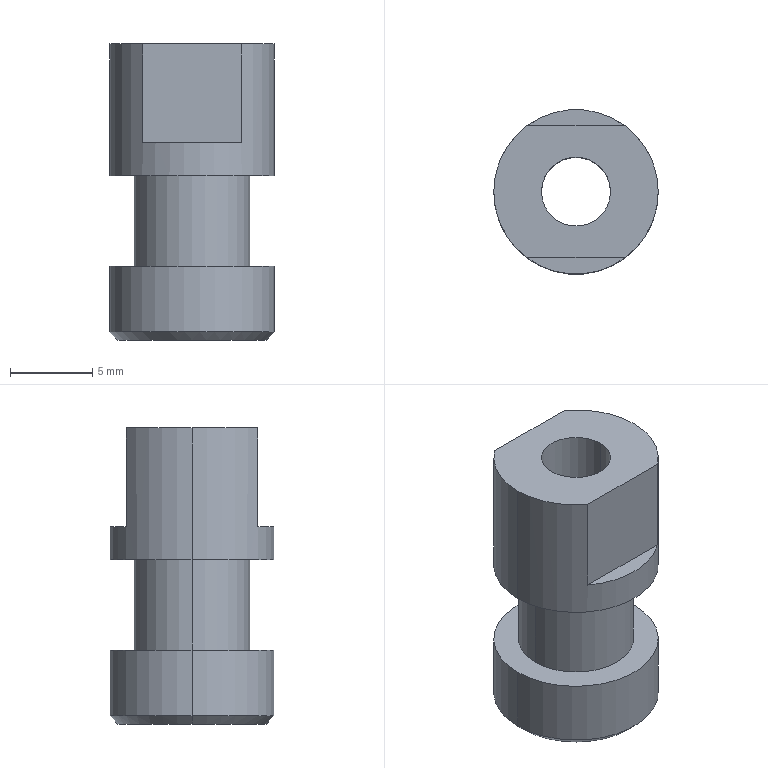Part | STEP file | 2079 Bag feed floating joint mounting | 1 solid | 18 faces | box 10 x 10 x 18 mm | volume 891.186 mm3 | cylinder 8 | plane 8 | cone 2 | commonest cylinder face diameters 10 x4 4.2 x2 7 x2
STEP:
#1=CARTESIAN_POINT('',(0.,0.,0.));
#2=DIRECTION('',(0.,0.,1.));
#3=DIRECTION('',(1.,0.,0.));
#4=AXIS2_PLACEMENT_3D('',#1,#2,#3);
#5=CARTESIAN_POINT('',(-4.5,0.,0.));
#6=VERTEX_POINT('',#5);
#7=CARTESIAN_POINT('',(4.5,0.,0.));
#8=VERTEX_POINT('',#7);
#9=CARTESIAN_POINT('',(0.,0.,0.));
#10=DIRECTION('',(0.,0.,-1.));
#11=DIRECTION('',(1.,0.,0.));
#12=AXIS2_PLACEMENT_3D('',#9,#10,#11);
#13=CIRCLE('',#12,4.5);
#14=CARTESIAN_POINT('',(0.,0.,0.5));
#15=DIRECTION('',(0.,0.,1.));
#16=DIRECTION('',(1.,0.,0.));
#17=AXIS2_PLACEMENT_3D('',#14,#15,#16);
#18=CONICAL_SURFACE('',#17,5.,0.7854);
#19=CARTESIAN_POINT('',(6.283,-0.5));
#20=DIRECTION('',(-1.,0.));
#21=VECTOR('',#20,1.);
#22=LINE('',#19,#21);
#23=(GEOMETRIC_REPRESENTATION_CONTEXT(2)PARAMETRIC_REPRESENTATION_CONTEXT()REPRESENTATION_CONTEXT('',''));
#24=DEFINITIONAL_REPRESENTATION('',(#22),#23);
#25=PCURVE('',#18,#24);
#26=CARTESIAN_POINT('',(0.,0.,0.));
#27=DIRECTION('',(0.,0.,1.));
#28=DIRECTION('',(1.,0.,0.));
#29=AXIS2_PLACEMENT_3D('',#26,#27,#28);
#30=PLANE('',#29);
#31=CARTESIAN_POINT('',(4.5,0.));
#32=CARTESIAN_POINT('',(4.5,-7.794));
#33=CARTESIAN_POINT('',(-2.25,-3.897));
#34=CARTESIAN_POINT('',(-9.,0.));
#35=CARTESIAN_POINT('',(-2.25,3.897));
#36=CARTESIAN_POINT('',(4.5,7.794));
#37=CARTESIAN_POINT('',(4.5,0.));
#38=(BOUNDED_CURVE()B_SPLINE_CURVE(2,(#31,#32,#33,#34,#35,#36,#37),.UNSPECIFIED.,.T.,.F.)B_SPLINE_CURVE_WITH_KNOTS((1,2,2,2,2,1),(-2.094,0.,2.094,4.189,6.283,8.378),.UNSPECIFIED.)CURVE()GEOMETRIC_REPRESENTATION_ITEM()RATIONAL_B_SPLINE_CURVE((1.,0.5,1.,0.5,1.,0.5,1.))REPRESENTATION_ITEM(''));
#39=(GEOMETRIC_REPRESENTATION_CONTEXT(2)PARAMETRIC_REPRESENTATION_CONTEXT()REPRESENTATION_CONTEXT('',''));
#40=DEFINITIONAL_REPRESENTATION('',(#38),#39);
#41=PCURVE('',#30,#40);
#42=SURFACE_CURVE('',#13,(#25,#41),.PCURVE_S1.);
#43=EDGE_CURVE('',#6,#8,#42,.T.);
#44=ORIENTED_EDGE('',*,*,#43,.F.);
#45=CARTESIAN_POINT('',(-5.,0.,0.5));
#46=VERTEX_POINT('',#45);
#47=CARTESIAN_POINT('',(-5.,0.,0.5));
#48=DIRECTION('',(-0.7071,0.,0.7071));
#49=VECTOR('',#48,1.);
#50=LINE('',#47,#49);
#51=CARTESIAN_POINT('',(3.142,0.));
#52=DIRECTION('',(0.,1.));
#53=VECTOR('',#52,1.);
#54=LINE('',#51,#53);
#55=(GEOMETRIC_REPRESENTATION_CONTEXT(2)PARAMETRIC_REPRESENTATION_CONTEXT()REPRESENTATION_CONTEXT('',''));
#56=DEFINITIONAL_REPRESENTATION('',(#54),#55);
#57=PCURVE('',#18,#56);
#58=CARTESIAN_POINT('',(0.,0.,0.5));
#59=DIRECTION('',(0.,0.,1.));
#60=DIRECTION('',(1.,0.,0.));
#61=AXIS2_PLACEMENT_3D('',#58,#59,#60);
#62=CONICAL_SURFACE('',#61,5.,0.7854);
#63=CARTESIAN_POINT('',(3.142,0.));
#64=DIRECTION('',(0.,1.));
#65=VECTOR('',#64,1.);
#66=LINE('',#63,#65);
#67=(GEOMETRIC_REPRESENTATION_CONTEXT(2)PARAMETRIC_REPRESENTATION_CONTEXT()REPRESENTATION_CONTEXT('',''));
#68=DEFINITIONAL_REPRESENTATION('',(#66),#67);
#69=PCURVE('',#62,#68);
#70=SURFACE_CURVE('',#50,(#57,#69),.PCURVE_S1.);
#71=EDGE_CURVE('',#6,#46,#70,.T.);
#72=ORIENTED_EDGE('',*,*,#71,.T.);
#73=CARTESIAN_POINT('',(5.,0.,0.5));
#74=VERTEX_POINT('',#73);
#75=CARTESIAN_POINT('',(0.,0.,0.5));
#76=DIRECTION('',(0.,0.,1.));
#77=DIRECTION('',(1.,0.,0.));
#78=AXIS2_PLACEMENT_3D('',#75,#76,#77);
#79=CIRCLE('',#78,5.);
#80=CARTESIAN_POINT('',(0.,0.));
#81=DIRECTION('',(1.,0.));
#82=VECTOR('',#81,1.);
#83=LINE('',#80,#82);
#84=(GEOMETRIC_REPRESENTATION_CONTEXT(2)PARAMETRIC_REPRESENTATION_CONTEXT()REPRESENTATION_CONTEXT('',''));
#85=DEFINITIONAL_REPRESENTATION('',(#83),#84);
#86=PCURVE('',#18,#85);
#87=CARTESIAN_POINT('',(0.,0.,4.5));
#88=DIRECTION('',(0.,0.,-1.));
#89=DIRECTION('',(-1.,0.,0.));
#90=AXIS2_PLACEMENT_3D('',#87,#88,#89);
#91=CYLINDRICAL_SURFACE('',#90,5.);
#92=CARTESIAN_POINT('',(3.142,4.));
#93=DIRECTION('',(-1.,0.));
#94=VECTOR('',#93,1.);
#95=LINE('',#92,#94);
#96=(GEOMETRIC_REPRESENTATION_CONTEXT(2)PARAMETRIC_REPRESENTATION_CONTEXT()REPRESENTATION_CONTEXT('',''));
#97=DEFINITIONAL_REPRESENTATION('',(#95),#96);
#98=PCURVE('',#91,#97);
#99=SURFACE_CURVE('',#79,(#86,#98),.PCURVE_S1.);
#100=EDGE_CURVE('',#74,#46,#99,.T.);
#101=ORIENTED_EDGE('',*,*,#100,.F.);
#102=CARTESIAN_POINT('',(5.,0.,0.5));
#103=DIRECTION('',(0.7071,0.,0.7071));
#104=VECTOR('',#103,1.);
#105=LINE('',#102,#104);
#106=CARTESIAN_POINT('',(0.,0.));
#107=DIRECTION('',(0.,1.));
#108=VECTOR('',#107,1.);
#109=LINE('',#106,#108);
#110=(GEOMETRIC_REPRESENTATION_CONTEXT(2)PARAMETRIC_REPRESENTATION_CONTEXT()REPRESENTATION_CONTEXT('',''));
#111=DEFINITIONAL_REPRESENTATION('',(#109),#110);
#112=PCURVE('',#18,#111);
#113=CARTESIAN_POINT('',(6.283,0.));
#114=DIRECTION('',(0.,1.));
#115=VECTOR('',#114,1.);
#116=LINE('',#113,#115);
#117=(GEOMETRIC_REPRESENTATION_CONTEXT(2)PARAMETRIC_REPRESENTATION_CONTEXT()REPRESENTATION_CONTEXT('',''));
#118=DEFINITIONAL_REPRESENTATION('',(#116),#117);
#119=PCURVE('',#62,#118);
#120=SURFACE_CURVE('',#105,(#112,#119),.PCURVE_S1.);
#121=EDGE_CURVE('',#8,#74,#120,.T.);
#122=ORIENTED_EDGE('',*,*,#121,.F.);
#123=EDGE_LOOP('',(#44,#72,#101,#122));
#124=FACE_BOUND('',#123,.T.);
#125=ADVANCED_FACE('',(#124),#18,.T.);
#126=CARTESIAN_POINT('',(2.1,0.,0.));
#127=VERTEX_POINT('',#126);
#128=CARTESIAN_POINT('',(2.1,0.,18.));
#129=VERTEX_POINT('',#128);
#130=CARTESIAN_POINT('',(2.1,0.,18.));
#131=DIRECTION('',(0.,0.,1.));
#132=VECTOR('',#131,1.);
#133=LINE('',#130,#132);
#134=CARTESIAN_POINT('',(0.,0.,18.));
#135=DIRECTION('',(0.,0.,1.));
#136=DIRECTION('',(1.,0.,0.));
#137=AXIS2_PLACEMENT_3D('',#134,#135,#136);
#138=CYLINDRICAL_SURFACE('',#137,2.1);
#139=CARTESIAN_POINT('',(6.283,0.));
#140=DIRECTION('',(0.,1.));
#141=VECTOR('',#140,1.);
#142=LINE('',#139,#141);
#143=(GEOMETRIC_REPRESENTATION_CONTEXT(2)PARAMETRIC_REPRESENTATION_CONTEXT()REPRESENTATION_CONTEXT('',''));
#144=DEFINITIONAL_REPRESENTATION('',(#142),#143);
#145=PCURVE('',#138,#144);
#146=CARTESIAN_POINT('',(0.,0.,18.));
#147=DIRECTION('',(0.,0.,1.));
#148=DIRECTION('',(1.,0.,0.));
#149=AXIS2_PLACEMENT_3D('',#146,#147,#148);
#150=CYLINDRICAL_SURFACE('',#149,2.1);
#151=CARTESIAN_POINT('',(0.,0.));
#152=DIRECTION('',(0.,1.));
#153=VECTOR('',#152,1.);
#154=LINE('',#151,#153);
#155=(GEOMETRIC_REPRESENTATION_CONTEXT(2)PARAMETRIC_REPRESENTATION_CONTEXT()REPRESENTATION_CONTEXT('',''));
#156=DEFINITIONAL_REPRESENTATION('',(#154),#155);
#157=PCURVE('',#150,#156);
#158=SURFACE_CURVE('',#133,(#145,#157),.PCURVE_S1.);
#159=EDGE_CURVE('',#127,#129,#158,.T.);
#160=ORIENTED_EDGE('',*,*,#159,.T.);
#161=CARTESIAN_POINT('',(-2.1,0.,18.));
#162=VERTEX_POINT('',#161);
#163=CARTESIAN_POINT('',(0.,0.,18.));
#164=DIRECTION('',(0.,0.,1.));
#165=DIRECTION('',(1.,0.,0.));
#166=AXIS2_PLACEMENT_3D('',#163,#164,#165);
#167=CIRCLE('',#166,2.1);
#168=CARTESIAN_POINT('',(0.,0.));
#169=DIRECTION('',(1.,0.));
#170=VECTOR('',#169,1.);
#171=LINE('',#168,#170);
#172=(GEOMETRIC_REPRESENTATION_CONTEXT(2)PARAMETRIC_REPRESENTATION_CONTEXT()REPRESENTATION_CONTEXT('',''));
#173=DEFINITIONAL_REPRESENTATION('',(#171),#172);
#174=PCURVE('',#138,#173);
#175=CARTESIAN_POINT('',(0.,0.,18.));
#176=DIRECTION('',(0.,0.,1.));
#177=DIRECTION('',(1.,0.,0.));
#178=AXIS2_PLACEMENT_3D('',#175,#176,#177);
#179=PLANE('',#178);
#180=CARTESIAN_POINT('',(0.,0.));
#181=DIRECTION('',(1.,0.));
#182=AXIS2_PLACEMENT_2D('',#180,#181);
#183=CIRCLE('',#182,2.1);
#184=(GEOMETRIC_REPRESENTATION_CONTEXT(2)PARAMETRIC_REPRESENTATION_CONTEXT()REPRESENTATION_CONTEXT('',''));
#185=DEFINITIONAL_REPRESENTATION('',(#183),#184);
#186=PCURVE('',#179,#185);
#187=SURFACE_CURVE('',#167,(#174,#186),.PCURVE_S1.);
#188=EDGE_CURVE('',#162,#129,#187,.T.);
#189=ORIENTED_EDGE('',*,*,#188,.F.);
#190=CARTESIAN_POINT('',(-2.1,0.,0.));
#191=VERTEX_POINT('',#190);
#192=CARTESIAN_POINT('',(-2.1,0.,18.));
#193=DIRECTION('',(0.,0.,1.));
#194=VECTOR('',#193,1.);
#195=LINE('',#192,#194);
#196=CARTESIAN_POINT('',(3.142,0.));
#197=DIRECTION('',(0.,1.));
#198=VECTOR('',#197,1.);
#199=LINE('',#196,#198);
#200=(GEOMETRIC_REPRESENTATION_CONTEXT(2)PARAMETRIC_REPRESENTATION_CONTEXT()REPRESENTATION_CONTEXT('',''));
#201=DEFINITIONAL_REPRESENTATION('',(#199),#200);
#202=PCURVE('',#138,#201);
#203=CARTESIAN_POINT('',(3.142,0.));
#204=DIRECTION('',(0.,1.));
#205=VECTOR('',#204,1.);
#206=LINE('',#203,#205);
#207=(GEOMETRIC_REPRESENTATION_CONTEXT(2)PARAMETRIC_REPRESENTATION_CONTEXT()REPRESENTATION_CONTEXT('',''));
#208=DEFINITIONAL_REPRESENTATION('',(#206),#207);
#209=PCURVE('',#150,#208);
#210=SURFACE_CURVE('',#195,(#202,#209),.PCURVE_S1.);
#211=EDGE_CURVE('',#191,#162,#210,.T.);
#212=ORIENTED_EDGE('',*,*,#211,.F.);
#213=CARTESIAN_POINT('',(0.,0.,0.));
#214=DIRECTION('',(0.,0.,1.));
#215=DIRECTION('',(1.,0.,0.));
#216=AXIS2_PLACEMENT_3D('',#213,#214,#215);
#217=CIRCLE('',#216,2.1);
#218=CARTESIAN_POINT('',(0.,-18.));
#219=DIRECTION('',(1.,0.));
#220=VECTOR('',#219,1.);
#221=LINE('',#218,#220);
#222=(GEOMETRIC_REPRESENTATION_CONTEXT(2)PARAMETRIC_REPRESENTATION_CONTEXT()REPRESENTATION_CONTEXT('',''));
#223=DEFINITIONAL_REPRESENTATION('',(#221),#222);
#224=PCURVE('',#138,#223);
#225=CARTESIAN_POINT('',(0.,0.));
#226=DIRECTION('',(1.,0.));
#227=AXIS2_PLACEMENT_2D('',#225,#226);
#228=CIRCLE('',#227,2.1);
#229=(GEOMETRIC_REPRESENTATION_CONTEXT(2)PARAMETRIC_REPRESENTATION_CONTEXT()REPRESENTATION_CONTEXT('',''));
#230=DEFINITIONAL_REPRESENTATION('',(#228),#229);
#231=PCURVE('',#30,#230);
#232=SURFACE_CURVE('',#217,(#224,#231),.PCURVE_S1.);
#233=EDGE_CURVE('',#191,#127,#232,.T.);
#234=ORIENTED_EDGE('',*,*,#233,.T.);
#235=EDGE_LOOP('',(#160,#189,#212,#234));
#236=FACE_BOUND('',#235,.F.);
#237=ADVANCED_FACE('',(#236),#138,.F.);
#238=CARTESIAN_POINT('',(5.,0.,18.));
#239=VERTEX_POINT('',#238);
#240=CARTESIAN_POINT('',(3.,4.,18.));
#241=VERTEX_POINT('',#240);
#242=CARTESIAN_POINT('',(0.,0.,18.));
#243=DIRECTION('',(0.,0.,1.));
#244=DIRECTION('',(1.,0.,0.));
#245=AXIS2_PLACEMENT_3D('',#242,#243,#244);
#246=CIRCLE('',#245,5.);
#247=CARTESIAN_POINT('',(0.,0.,18.));
#248=DIRECTION('',(0.,0.,-1.));
#249=DIRECTION('',(-1.,0.,0.));
#250=AXIS2_PLACEMENT_3D('',#247,#248,#249);
#251=CYLINDRICAL_SURFACE('',#250,5.);
#252=CARTESIAN_POINT('',(3.142,0.));
#253=DIRECTION('',(-1.,0.));
#254=VECTOR('',#253,1.);
#255=LINE('',#252,#254);
#256=(GEOMETRIC_REPRESENTATION_CONTEXT(2)PARAMETRIC_REPRESENTATION_CONTEXT()REPRESENTATION_CONTEXT('',''));
#257=DEFINITIONAL_REPRESENTATION('',(#255),#256);
#258=PCURVE('',#251,#257);
#259=CARTESIAN_POINT('',(0.,0.));
#260=DIRECTION('',(1.,0.));
#261=AXIS2_PLACEMENT_2D('',#259,#260);
#262=CIRCLE('',#261,5.);
#263=(GEOMETRIC_REPRESENTATION_CONTEXT(2)PARAMETRIC_REPRESENTATION_CONTEXT()REPRESENTATION_CONTEXT('',''));
#264=DEFINITIONAL_REPRESENTATION('',(#262),#263);
#265=PCURVE('',#179,#264);
#266=SURFACE_CURVE('',#246,(#258,#265),.PCURVE_S1.);
#267=EDGE_CURVE('',#239,#241,#266,.T.);
#268=ORIENTED_EDGE('',*,*,#267,.F.);
#269=CARTESIAN_POINT('',(5.,0.,10.));
#270=VERTEX_POINT('',#269);
#271=CARTESIAN_POINT('',(5.,0.,18.));
#272=DIRECTION('',(0.,0.,-1.));
#273=VECTOR('',#272,1.);
#274=LINE('',#271,#273);
#275=CARTESIAN_POINT('',(3.142,0.));
#276=DIRECTION('',(0.,1.));
#277=VECTOR('',#276,1.);
#278=LINE('',#275,#277);
#279=(GEOMETRIC_REPRESENTATION_CONTEXT(2)PARAMETRIC_REPRESENTATION_CONTEXT()REPRESENTATION_CONTEXT('',''));
#280=DEFINITIONAL_REPRESENTATION('',(#278),#279);
#281=PCURVE('',#251,#280);
#282=CARTESIAN_POINT('',(0.,0.,18.));
#283=DIRECTION('',(0.,0.,-1.));
#284=DIRECTION('',(-1.,0.,0.));
#285=AXIS2_PLACEMENT_3D('',#282,#283,#284);
#286=CYLINDRICAL_SURFACE('',#285,5.);
#287=CARTESIAN_POINT('',(3.142,0.));
#288=DIRECTION('',(0.,1.));
#289=VECTOR('',#288,1.);
#290=LINE('',#287,#289);
#291=(GEOMETRIC_REPRESENTATION_CONTEXT(2)PARAMETRIC_REPRESENTATION_CONTEXT()REPRESENTATION_CONTEXT('',''));
#292=DEFINITIONAL_REPRESENTATION('',(#290),#291);
#293=PCURVE('',#286,#292);
#294=SURFACE_CURVE('',#274,(#281,#293),.PCURVE_S1.);
#295=EDGE_CURVE('',#239,#270,#294,.T.);
#296=ORIENTED_EDGE('',*,*,#295,.T.);
#297=CARTESIAN_POINT('',(-5.,0.,10.));
#298=VERTEX_POINT('',#297);
#299=CARTESIAN_POINT('',(0.,0.,10.));
#300=DIRECTION('',(0.,0.,1.));
#301=DIRECTION('',(1.,0.,0.));
#302=AXIS2_PLACEMENT_3D('',#299,#300,#301);
#303=CIRCLE('',#302,5.);
#304=CARTESIAN_POINT('',(3.142,8.));
#305=DIRECTION('',(-1.,0.));
#306=VECTOR('',#305,1.);
#307=LINE('',#304,#306);
#308=(GEOMETRIC_REPRESENTATION_CONTEXT(2)PARAMETRIC_REPRESENTATION_CONTEXT()REPRESENTATION_CONTEXT('',''));
#309=DEFINITIONAL_REPRESENTATION('',(#307),#308);
#310=PCURVE('',#251,#309);
#311=CARTESIAN_POINT('',(0.,0.,10.));
#312=DIRECTION('',(0.,0.,1.));
#313=DIRECTION('',(1.,0.,0.));
#314=AXIS2_PLACEMENT_3D('',#311,#312,#313);
#315=PLANE('',#314);
#316=CARTESIAN_POINT('',(0.,0.));
#317=DIRECTION('',(1.,0.));
#318=AXIS2_PLACEMENT_2D('',#316,#317);
#319=CIRCLE('',#318,5.);
#320=(GEOMETRIC_REPRESENTATION_CONTEXT(2)PARAMETRIC_REPRESENTATION_CONTEXT()REPRESENTATION_CONTEXT('',''));
#321=DEFINITIONAL_REPRESENTATION('',(#319),#320);
#322=PCURVE('',#315,#321);
#323=SURFACE_CURVE('',#303,(#310,#322),.PCURVE_S1.);
#324=EDGE_CURVE('',#270,#298,#323,.T.);
#325=ORIENTED_EDGE('',*,*,#324,.T.);
#326=CARTESIAN_POINT('',(-5.,0.,18.));
#327=VERTEX_POINT('',#326);
#328=CARTESIAN_POINT('',(-5.,0.,18.));
#329=DIRECTION('',(0.,0.,-1.));
#330=VECTOR('',#329,1.);
#331=LINE('',#328,#330);
#332=CARTESIAN_POINT('',(0.,0.));
#333=DIRECTION('',(0.,1.));
#334=VECTOR('',#333,1.);
#335=LINE('',#332,#334);
#336=(GEOMETRIC_REPRESENTATION_CONTEXT(2)PARAMETRIC_REPRESENTATION_CONTEXT()REPRESENTATION_CONTEXT('',''));
#337=DEFINITIONAL_REPRESENTATION('',(#335),#336);
#338=PCURVE('',#251,#337);
#339=CARTESIAN_POINT('',(6.283,0.));
#340=DIRECTION('',(0.,1.));
#341=VECTOR('',#340,1.);
#342=LINE('',#339,#341);
#343=(GEOMETRIC_REPRESENTATION_CONTEXT(2)PARAMETRIC_REPRESENTATION_CONTEXT()REPRESENTATION_CONTEXT('',''));
#344=DEFINITIONAL_REPRESENTATION('',(#342),#343);
#345=PCURVE('',#286,#344);
#346=SURFACE_CURVE('',#331,(#338,#345),.PCURVE_S1.);
#347=EDGE_CURVE('',#327,#298,#346,.T.);
#348=ORIENTED_EDGE('',*,*,#347,.F.);
#349=CARTESIAN_POINT('',(-3.,4.,18.));
#350=VERTEX_POINT('',#349);
#351=CARTESIAN_POINT('',(0.,0.,18.));
#352=DIRECTION('',(0.,0.,1.));
#353=DIRECTION('',(1.,0.,0.));
#354=AXIS2_PLACEMENT_3D('',#351,#352,#353);
#355=CIRCLE('',#354,5.);
#356=CARTESIAN_POINT('',(3.142,0.));
#357=DIRECTION('',(-1.,0.));
#358=VECTOR('',#357,1.);
#359=LINE('',#356,#358);
#360=(GEOMETRIC_REPRESENTATION_CONTEXT(2)PARAMETRIC_REPRESENTATION_CONTEXT()REPRESENTATION_CONTEXT('',''));
#361=DEFINITIONAL_REPRESENTATION('',(#359),#360);
#362=PCURVE('',#251,#361);
#363=CARTESIAN_POINT('',(0.,0.));
#364=DIRECTION('',(1.,0.));
#365=AXIS2_PLACEMENT_2D('',#363,#364);
#366=CIRCLE('',#365,5.);
#367=(GEOMETRIC_REPRESENTATION_CONTEXT(2)PARAMETRIC_REPRESENTATION_CONTEXT()REPRESENTATION_CONTEXT('',''));
#368=DEFINITIONAL_REPRESENTATION('',(#366),#367);
#369=PCURVE('',#179,#368);
#370=SURFACE_CURVE('',#355,(#362,#369),.PCURVE_S1.);
#371=EDGE_CURVE('',#350,#327,#370,.T.);
#372=ORIENTED_EDGE('',*,*,#371,.F.);
#373=CARTESIAN_POINT('',(-3.,4.,12.));
#374=VERTEX_POINT('',#373);
#375=CARTESIAN_POINT('',(-3.,4.,18.));
#376=DIRECTION('',(0.,0.,-1.));
#377=VECTOR('',#376,1.);
#378=LINE('',#375,#377);
#379=CARTESIAN_POINT('',(0.9273,0.));
#380=DIRECTION('',(0.,1.));
#381=VECTOR('',#380,1.);
#382=LINE('',#379,#381);
#383=(GEOMETRIC_REPRESENTATION_CONTEXT(2)PARAMETRIC_REPRESENTATION_CONTEXT()REPRESENTATION_CONTEXT('',''));
#384=DEFINITIONAL_REPRESENTATION('',(#382),#383);
#385=PCURVE('',#251,#384);
#386=CARTESIAN_POINT('',(5.719,4.,12.));
#387=DIRECTION('',(0.,-1.,0.));
#388=DIRECTION('',(1.,0.,0.));
#389=AXIS2_PLACEMENT_3D('',#386,#387,#388);
#390=PLANE('',#389);
#391=CARTESIAN_POINT('',(-8.719,6.));
#392=DIRECTION('',(0.,-1.));
#393=VECTOR('',#392,1.);
#394=LINE('',#391,#393);
#395=(GEOMETRIC_REPRESENTATION_CONTEXT(2)PARAMETRIC_REPRESENTATION_CONTEXT()REPRESENTATION_CONTEXT('',''));
#396=DEFINITIONAL_REPRESENTATION('',(#394),#395);
#397=PCURVE('',#390,#396);
#398=SURFACE_CURVE('',#378,(#385,#397),.PCURVE_S1.);
#399=EDGE_CURVE('',#350,#374,#398,.T.);
#400=ORIENTED_EDGE('',*,*,#399,.T.);
#401=CARTESIAN_POINT('',(3.,4.,12.));
#402=VERTEX_POINT('',#401);
#403=CARTESIAN_POINT('',(0.,0.,12.));
#404=DIRECTION('',(0.,0.,1.));
#405=DIRECTION('',(1.,0.,0.));
#406=AXIS2_PLACEMENT_3D('',#403,#404,#405);
#407=CIRCLE('',#406,5.);
#408=CARTESIAN_POINT('',(3.142,6.));
#409=DIRECTION('',(-1.,0.));
#410=VECTOR('',#409,1.);
#411=LINE('',#408,#410);
#412=(GEOMETRIC_REPRESENTATION_CONTEXT(2)PARAMETRIC_REPRESENTATION_CONTEXT()REPRESENTATION_CONTEXT('',''));
#413=DEFINITIONAL_REPRESENTATION('',(#411),#412);
#414=PCURVE('',#251,#413);
#415=CARTESIAN_POINT('',(0.,0.,12.));
#416=DIRECTION('',(0.,0.,1.));
#417=DIRECTION('',(1.,0.,0.));
#418=AXIS2_PLACEMENT_3D('',#415,#416,#417);
#419=PLANE('',#418);
#420=CARTESIAN_POINT('',(0.,0.));
#421=DIRECTION('',(1.,0.));
#422=AXIS2_PLACEMENT_2D('',#420,#421);
#423=CIRCLE('',#422,5.);
#424=(GEOMETRIC_REPRESENTATION_CONTEXT(2)PARAMETRIC_REPRESENTATION_CONTEXT()REPRESENTATION_CONTEXT('',''));
#425=DEFINITIONAL_REPRESENTATION('',(#423),#424);
#426=PCURVE('',#419,#425);
#427=SURFACE_CURVE('',#407,(#414,#426),.PCURVE_S1.);
#428=EDGE_CURVE('',#402,#374,#427,.T.);
#429=ORIENTED_EDGE('',*,*,#428,.F.);
#430=CARTESIAN_POINT('',(3.,4.,18.));
#431=DIRECTION('',(0.,0.,1.));
#432=VECTOR('',#431,1.);
#433=LINE('',#430,#432);
#434=CARTESIAN_POINT('',(2.214,0.));
#435=DIRECTION('',(0.,-1.));
#436=VECTOR('',#435,1.);
#437=LINE('',#434,#436);
#438=(GEOMETRIC_REPRESENTATION_CONTEXT(2)PARAMETRIC_REPRESENTATION_CONTEXT()REPRESENTATION_CONTEXT('',''));
#439=DEFINITIONAL_REPRESENTATION('',(#437),#438);
#440=PCURVE('',#251,#439);
#441=CARTESIAN_POINT('',(-2.719,6.));
#442=DIRECTION('',(0.,1.));
#443=VECTOR('',#442,1.);
#444=LINE('',#441,#443);
#445=(GEOMETRIC_REPRESENTATION_CONTEXT(2)PARAMETRIC_REPRESENTATION_CONTEXT()REPRESENTATION_CONTEXT('',''));
#446=DEFINITIONAL_REPRESENTATION('',(#444),#445);
#447=PCURVE('',#390,#446);
#448=SURFACE_CURVE('',#433,(#440,#447),.PCURVE_S1.);
#449=EDGE_CURVE('',#402,#241,#448,.T.);
#450=ORIENTED_EDGE('',*,*,#449,.T.);
#451=EDGE_LOOP('',(#268,#296,#325,#348,#372,#400,#429,#450));
#452=FACE_BOUND('',#451,.T.);
#453=ADVANCED_FACE('',(#452),#251,.T.);
#454=CARTESIAN_POINT('',(3.5,0.,10.));
#455=VERTEX_POINT('',#454);
#456=CARTESIAN_POINT('',(-3.5,0.,10.));
#457=VERTEX_POINT('',#456);
#458=CARTESIAN_POINT('',(0.,0.,10.));
#459=DIRECTION('',(0.,0.,1.));
#460=DIRECTION('',(1.,0.,0.));
#461=AXIS2_PLACEMENT_3D('',#458,#459,#460);
#462=CIRCLE('',#461,3.5);
#463=CARTESIAN_POINT('',(0.,0.,10.));
#464=DIRECTION('',(0.,0.,-1.));
#465=DIRECTION('',(-1.,0.,0.));
#466=AXIS2_PLACEMENT_3D('',#463,#464,#465);
#467=CYLINDRICAL_SURFACE('',#466,3.5);
#468=CARTESIAN_POINT('',(3.142,0.));
#469=DIRECTION('',(-1.,0.));
#470=VECTOR('',#469,1.);
#471=LINE('',#468,#470);
#472=(GEOMETRIC_REPRESENTATION_CONTEXT(2)PARAMETRIC_REPRESENTATION_CONTEXT()REPRESENTATION_CONTEXT('',''));
#473=DEFINITIONAL_REPRESENTATION('',(#471),#472);
#474=PCURVE('',#467,#473);
#475=CARTESIAN_POINT('',(0.,0.));
#476=DIRECTION('',(1.,0.));
#477=AXIS2_PLACEMENT_2D('',#475,#476);
#478=CIRCLE('',#477,3.5);
#479=(GEOMETRIC_REPRESENTATION_CONTEXT(2)PARAMETRIC_REPRESENTATION_CONTEXT()REPRESENTATION_CONTEXT('',''));
#480=DEFINITIONAL_REPRESENTATION('',(#478),#479);
#481=PCURVE('',#315,#480);
#482=SURFACE_CURVE('',#462,(#474,#481),.PCURVE_S1.);
#483=EDGE_CURVE('',#455,#457,#482,.T.);
#484=ORIENTED_EDGE('',*,*,#483,.F.);
#485=CARTESIAN_POINT('',(3.5,0.,4.5));
#486=VERTEX_POINT('',#485);
#487=CARTESIAN_POINT('',(3.5,0.,10.));
#488=DIRECTION('',(0.,0.,-1.));
#489=VECTOR('',#488,1.);
#490=LINE('',#487,#489);
#491=CARTESIAN_POINT('',(3.142,0.));
#492=DIRECTION('',(0.,1.));
#493=VECTOR('',#492,1.);
#494=LINE('',#491,#493);
#495=(GEOMETRIC_REPRESENTATION_CONTEXT(2)PARAMETRIC_REPRESENTATION_CONTEXT()REPRESENTATION_CONTEXT('',''));
#496=DEFINITIONAL_REPRESENTATION('',(#494),#495);
#497=PCURVE('',#467,#496);
#498=CARTESIAN_POINT('',(0.,0.,10.));
#499=DIRECTION('',(0.,0.,-1.));
#500=DIRECTION('',(-1.,0.,0.));
#501=AXIS2_PLACEMENT_3D('',#498,#499,#500);
#502=CYLINDRICAL_SURFACE('',#501,3.5);
#503=CARTESIAN_POINT('',(3.142,0.));
#504=DIRECTION('',(0.,1.));
#505=VECTOR('',#504,1.);
#506=LINE('',#503,#505);
#507=(GEOMETRIC_REPRESENTATION_CONTEXT(2)PARAMETRIC_REPRESENTATION_CONTEXT()REPRESENTATION_CONTEXT('',''));
#508=DEFINITIONAL_REPRESENTATION('',(#506),#507);
#509=PCURVE('',#502,#508);
#510=SURFACE_CURVE('',#490,(#497,#509),.PCURVE_S1.);
#511=EDGE_CURVE('',#455,#486,#510,.T.);
#512=ORIENTED_EDGE('',*,*,#511,.T.);
#513=CARTESIAN_POINT('',(-3.5,0.,4.5));
#514=VERTEX_POINT('',#513);
#515=CARTESIAN_POINT('',(0.,0.,4.5));
#516=DIRECTION('',(0.,0.,1.));
#517=DIRECTION('',(1.,0.,0.));
#518=AXIS2_PLACEMENT_3D('',#515,#516,#517);
#519=CIRCLE('',#518,3.5);
#520=CARTESIAN_POINT('',(3.142,5.5));
#521=DIRECTION('',(-1.,0.));
#522=VECTOR('',#521,1.);
#523=LINE('',#520,#522);
#524=(GEOMETRIC_REPRESENTATION_CONTEXT(2)PARAMETRIC_REPRESENTATION_CONTEXT()REPRESENTATION_CONTEXT('',''));
#525=DEFINITIONAL_REPRESENTATION('',(#523),#524);
#526=PCURVE('',#467,#525);
#527=CARTESIAN_POINT('',(0.,0.,4.5));
#528=DIRECTION('',(0.,0.,1.));
#529=DIRECTION('',(1.,0.,0.));
#530=AXIS2_PLACEMENT_3D('',#527,#528,#529);
#531=PLANE('',#530);
#532=CARTESIAN_POINT('',(0.,0.));
#533=DIRECTION('',(1.,0.));
#534=AXIS2_PLACEMENT_2D('',#532,#533);
#535=CIRCLE('',#534,3.5);
#536=(GEOMETRIC_REPRESENTATION_CONTEXT(2)PARAMETRIC_REPRESENTATION_CONTEXT()REPRESENTATION_CONTEXT('',''));
#537=DEFINITIONAL_REPRESENTATION('',(#535),#536);
#538=PCURVE('',#531,#537);
#539=SURFACE_CURVE('',#519,(#526,#538),.PCURVE_S1.);
#540=EDGE_CURVE('',#486,#514,#539,.T.);
#541=ORIENTED_EDGE('',*,*,#540,.T.);
#542=CARTESIAN_POINT('',(-3.5,0.,10.));
#543=DIRECTION('',(0.,0.,-1.));
#544=VECTOR('',#543,1.);
#545=LINE('',#542,#544);
#546=CARTESIAN_POINT('',(0.,0.));
#547=DIRECTION('',(0.,1.));
#548=VECTOR('',#547,1.);
#549=LINE('',#546,#548);
#550=(GEOMETRIC_REPRESENTATION_CONTEXT(2)PARAMETRIC_REPRESENTATION_CONTEXT()REPRESENTATION_CONTEXT('',''));
#551=DEFINITIONAL_REPRESENTATION('',(#549),#550);
#552=PCURVE('',#467,#551);
#553=CARTESIAN_POINT('',(6.283,0.));
#554=DIRECTION('',(0.,1.));
#555=VECTOR('',#554,1.);
#556=LINE('',#553,#555);
#557=(GEOMETRIC_REPRESENTATION_CONTEXT(2)PARAMETRIC_REPRESENTATION_CONTEXT()REPRESENTATION_CONTEXT('',''));
#558=DEFINITIONAL_REPRESENTATION('',(#556),#557);
#559=PCURVE('',#502,#558);
#560=SURFACE_CURVE('',#545,(#552,#559),.PCURVE_S1.);
#561=EDGE_CURVE('',#457,#514,#560,.T.);
#562=ORIENTED_EDGE('',*,*,#561,.F.);
#563=EDGE_LOOP('',(#484,#512,#541,#562));
#564=FACE_BOUND('',#563,.T.);
#565=ADVANCED_FACE('',(#564),#467,.T.);
#566=CARTESIAN_POINT('',(5.,0.,4.5));
#567=VERTEX_POINT('',#566);
#568=CARTESIAN_POINT('',(-5.,0.,4.5));
#569=VERTEX_POINT('',#568);
#570=CARTESIAN_POINT('',(0.,0.,4.5));
#571=DIRECTION('',(0.,0.,1.));
#572=DIRECTION('',(1.,0.,0.));
#573=AXIS2_PLACEMENT_3D('',#570,#571,#572);
#574=CIRCLE('',#573,5.);
#575=CARTESIAN_POINT('',(3.142,0.));
#576=DIRECTION('',(-1.,0.));
#577=VECTOR('',#576,1.);
#578=LINE('',#575,#577);
#579=(GEOMETRIC_REPRESENTATION_CONTEXT(2)PARAMETRIC_REPRESENTATION_CONTEXT()REPRESENTATION_CONTEXT('',''));
#580=DEFINITIONAL_REPRESENTATION('',(#578),#579);
#581=PCURVE('',#91,#580);
#582=CARTESIAN_POINT('',(0.,0.));
#583=DIRECTION('',(1.,0.));
#584=AXIS2_PLACEMENT_2D('',#582,#583);
#585=CIRCLE('',#584,5.);
#586=(GEOMETRIC_REPRESENTATION_CONTEXT(2)PARAMETRIC_REPRESENTATION_CONTEXT()REPRESENTATION_CONTEXT('',''));
#587=DEFINITIONAL_REPRESENTATION('',(#585),#586);
#588=PCURVE('',#531,#587);
#589=SURFACE_CURVE('',#574,(#581,#588),.PCURVE_S1.);
#590=EDGE_CURVE('',#567,#569,#589,.T.);
#591=ORIENTED_EDGE('',*,*,#590,.F.);
#592=CARTESIAN_POINT('',(5.,0.,4.5));
#593=DIRECTION('',(0.,0.,-1.));
#594=VECTOR('',#593,1.);
#595=LINE('',#592,#594);
#596=CARTESIAN_POINT('',(3.142,0.));
#597=DIRECTION('',(0.,1.));
#598=VECTOR('',#597,1.);
#599=LINE('',#596,#598);
#600=(GEOMETRIC_REPRESENTATION_CONTEXT(2)PARAMETRIC_REPRESENTATION_CONTEXT()REPRESENTATION_CONTEXT('',''));
#601=DEFINITIONAL_REPRESENTATION('',(#599),#600);
#602=PCURVE('',#91,#601);
#603=CARTESIAN_POINT('',(0.,0.,4.5));
#604=DIRECTION('',(0.,0.,-1.));
#605=DIRECTION('',(-1.,0.,0.));
#606=AXIS2_PLACEMENT_3D('',#603,#604,#605);
#607=CYLINDRICAL_SURFACE('',#606,5.);
#608=CARTESIAN_POINT('',(3.142,0.));
#609=DIRECTION('',(0.,1.));
#610=VECTOR('',#609,1.);
#611=LINE('',#608,#610);
#612=(GEOMETRIC_REPRESENTATION_CONTEXT(2)PARAMETRIC_REPRESENTATION_CONTEXT()REPRESENTATION_CONTEXT('',''));
#613=DEFINITIONAL_REPRESENTATION('',(#611),#612);
#614=PCURVE('',#607,#613);
#615=SURFACE_CURVE('',#595,(#602,#614),.PCURVE_S1.);
#616=EDGE_CURVE('',#567,#74,#615,.T.);
#617=ORIENTED_EDGE('',*,*,#616,.T.);
#618=ORIENTED_EDGE('',*,*,#100,.T.);
#619=CARTESIAN_POINT('',(-5.,0.,4.5));
#620=DIRECTION('',(0.,0.,-1.));
#621=VECTOR('',#620,1.);
#622=LINE('',#619,#621);
#623=CARTESIAN_POINT('',(0.,0.));
#624=DIRECTION('',(0.,1.));
#625=VECTOR('',#624,1.);
#626=LINE('',#623,#625);
#627=(GEOMETRIC_REPRESENTATION_CONTEXT(2)PARAMETRIC_REPRESENTATION_CONTEXT()REPRESENTATION_CONTEXT('',''));
#628=DEFINITIONAL_REPRESENTATION('',(#626),#627);
#629=PCURVE('',#91,#628);
#630=CARTESIAN_POINT('',(6.283,0.));
#631=DIRECTION('',(0.,1.));
#632=VECTOR('',#631,1.);
#633=LINE('',#630,#632);
#634=(GEOMETRIC_REPRESENTATION_CONTEXT(2)PARAMETRIC_REPRESENTATION_CONTEXT()REPRESENTATION_CONTEXT('',''));
#635=DEFINITIONAL_REPRESENTATION('',(#633),#634);
#636=PCURVE('',#607,#635);
#637=SURFACE_CURVE('',#622,(#629,#636),.PCURVE_S1.);
#638=EDGE_CURVE('',#569,#46,#637,.T.);
#639=ORIENTED_EDGE('',*,*,#638,.F.);
#640=EDGE_LOOP('',(#591,#617,#618,#639));
#641=FACE_BOUND('',#640,.T.);
#642=ADVANCED_FACE('',(#641),#91,.T.);
#643=CARTESIAN_POINT('',(0.,0.,4.5));
#644=DIRECTION('',(0.,0.,1.));
#645=DIRECTION('',(1.,0.,0.));
#646=AXIS2_PLACEMENT_3D('',#643,#644,#645);
#647=CIRCLE('',#646,5.);
#648=CARTESIAN_POINT('',(0.,0.));
#649=DIRECTION('',(1.,0.));
#650=AXIS2_PLACEMENT_2D('',#648,#649);
#651=CIRCLE('',#650,5.);
#652=(GEOMETRIC_REPRESENTATION_CONTEXT(2)PARAMETRIC_REPRESENTATION_CONTEXT()REPRESENTATION_CONTEXT('',''));
#653=DEFINITIONAL_REPRESENTATION('',(#651),#652);
#654=PCURVE('',#531,#653);
#655=CARTESIAN_POINT('',(9.425,0.));
#656=DIRECTION('',(-1.,0.));
#657=VECTOR('',#656,1.);
#658=LINE('',#655,#657);
#659=(GEOMETRIC_REPRESENTATION_CONTEXT(2)PARAMETRIC_REPRESENTATION_CONTEXT()REPRESENTATION_CONTEXT('',''));
#660=DEFINITIONAL_REPRESENTATION('',(#658),#659);
#661=PCURVE('',#607,#660);
#662=SURFACE_CURVE('',#647,(#654,#661),.PCURVE_S1.);
#663=EDGE_CURVE('',#569,#567,#662,.T.);
#664=ORIENTED_EDGE('',*,*,#663,.T.);
#665=ORIENTED_EDGE('',*,*,#590,.T.);
#666=EDGE_LOOP('',(#664,#665));
#667=FACE_BOUND('',#666,.T.);
#668=CARTESIAN_POINT('',(0.,0.,4.5));
#669=DIRECTION('',(0.,0.,1.));
#670=DIRECTION('',(1.,0.,0.));
#671=AXIS2_PLACEMENT_3D('',#668,#669,#670);
#672=CIRCLE('',#671,3.5);
#673=CARTESIAN_POINT('',(0.,0.));
#674=DIRECTION('',(1.,0.));
#675=AXIS2_PLACEMENT_2D('',#673,#674);
#676=CIRCLE('',#675,3.5);
#677=(GEOMETRIC_REPRESENTATION_CONTEXT(2)PARAMETRIC_REPRESENTATION_CONTEXT()REPRESENTATION_CONTEXT('',''));
#678=DEFINITIONAL_REPRESENTATION('',(#676),#677);
#679=PCURVE('',#531,#678);
#680=CARTESIAN_POINT('',(9.425,5.5));
#681=DIRECTION('',(-1.,0.));
#682=VECTOR('',#681,1.);
#683=LINE('',#680,#682);
#684=(GEOMETRIC_REPRESENTATION_CONTEXT(2)PARAMETRIC_REPRESENTATION_CONTEXT()REPRESENTATION_CONTEXT('',''));
#685=DEFINITIONAL_REPRESENTATION('',(#683),#684);
#686=PCURVE('',#502,#685);
#687=SURFACE_CURVE('',#672,(#679,#686),.PCURVE_S1.);
#688=EDGE_CURVE('',#514,#486,#687,.T.);
#689=ORIENTED_EDGE('',*,*,#688,.F.);
#690=ORIENTED_EDGE('',*,*,#540,.F.);
#691=EDGE_LOOP('',(#689,#690));
#692=FACE_BOUND('',#691,.T.);
#693=ADVANCED_FACE('',(#667,#692),#531,.T.);
#694=ORIENTED_EDGE('',*,*,#616,.F.);
#695=ORIENTED_EDGE('',*,*,#663,.F.);
#696=ORIENTED_EDGE('',*,*,#638,.T.);
#697=CARTESIAN_POINT('',(0.,0.,0.5));
#698=DIRECTION('',(0.,0.,1.));
#699=DIRECTION('',(1.,0.,0.));
#700=AXIS2_PLACEMENT_3D('',#697,#698,#699);
#701=CIRCLE('',#700,5.);
#702=CARTESIAN_POINT('',(9.425,4.));
#703=DIRECTION('',(-1.,0.));
#704=VECTOR('',#703,1.);
#705=LINE('',#702,#704);
#706=(GEOMETRIC_REPRESENTATION_CONTEXT(2)PARAMETRIC_REPRESENTATION_CONTEXT()REPRESENTATION_CONTEXT('',''));
#707=DEFINITIONAL_REPRESENTATION('',(#705),#706);
#708=PCURVE('',#607,#707);
#709=CARTESIAN_POINT('',(0.,0.));
#710=DIRECTION('',(1.,0.));
#711=VECTOR('',#710,1.);
#712=LINE('',#709,#711);
#713=(GEOMETRIC_REPRESENTATION_CONTEXT(2)PARAMETRIC_REPRESENTATION_CONTEXT()REPRESENTATION_CONTEXT('',''));
#714=DEFINITIONAL_REPRESENTATION('',(#712),#713);
#715=PCURVE('',#62,#714);
#716=SURFACE_CURVE('',#701,(#708,#715),.PCURVE_S1.);
#717=EDGE_CURVE('',#46,#74,#716,.T.);
#718=ORIENTED_EDGE('',*,*,#717,.T.);
#719=EDGE_LOOP('',(#694,#695,#696,#718));
#720=FACE_BOUND('',#719,.T.);
#721=ADVANCED_FACE('',(#720),#607,.T.);
#722=CARTESIAN_POINT('',(0.,0.,0.));
#723=DIRECTION('',(0.,0.,-1.));
#724=DIRECTION('',(1.,0.,0.));
#725=AXIS2_PLACEMENT_3D('',#722,#723,#724);
#726=CIRCLE('',#725,4.5);
#727=CARTESIAN_POINT('',(4.5,0.));
#728=CARTESIAN_POINT('',(4.5,-7.794));
#729=CARTESIAN_POINT('',(-2.25,-3.897));
#730=CARTESIAN_POINT('',(-9.,0.));
#731=CARTESIAN_POINT('',(-2.25,3.897));
#732=CARTESIAN_POINT('',(4.5,7.794));
#733=CARTESIAN_POINT('',(4.5,0.));
#734=(BOUNDED_CURVE()B_SPLINE_CURVE(2,(#727,#728,#729,#730,#731,#732,#733),.UNSPECIFIED.,.T.,.F.)B_SPLINE_CURVE_WITH_KNOTS((1,2,2,2,2,1),(-2.094,0.,2.094,4.189,6.283,8.378),.UNSPECIFIED.)CURVE()GEOMETRIC_REPRESENTATION_ITEM()RATIONAL_B_SPLINE_CURVE((1.,0.5,1.,0.5,1.,0.5,1.))REPRESENTATION_ITEM(''));
#735=(GEOMETRIC_REPRESENTATION_CONTEXT(2)PARAMETRIC_REPRESENTATION_CONTEXT()REPRESENTATION_CONTEXT('',''));
#736=DEFINITIONAL_REPRESENTATION('',(#734),#735);
#737=PCURVE('',#30,#736);
#738=CARTESIAN_POINT('',(6.283,-0.5));
#739=DIRECTION('',(-1.,0.));
#740=VECTOR('',#739,1.);
#741=LINE('',#738,#740);
#742=(GEOMETRIC_REPRESENTATION_CONTEXT(2)PARAMETRIC_REPRESENTATION_CONTEXT()REPRESENTATION_CONTEXT('',''));
#743=DEFINITIONAL_REPRESENTATION('',(#741),#742);
#744=PCURVE('',#62,#743);
#745=SURFACE_CURVE('',#726,(#737,#744),.PCURVE_S1.);
#746=EDGE_CURVE('',#8,#6,#745,.T.);
#747=ORIENTED_EDGE('',*,*,#746,.T.);
#748=ORIENTED_EDGE('',*,*,#43,.T.);
#749=EDGE_LOOP('',(#747,#748));
#750=FACE_BOUND('',#749,.T.);
#751=CARTESIAN_POINT('',(0.,0.,0.));
#752=DIRECTION('',(0.,0.,1.));
#753=DIRECTION('',(1.,0.,0.));
#754=AXIS2_PLACEMENT_3D('',#751,#752,#753);
#755=CIRCLE('',#754,2.1);
#756=CARTESIAN_POINT('',(0.,0.));
#757=DIRECTION('',(1.,0.));
#758=AXIS2_PLACEMENT_2D('',#756,#757);
#759=CIRCLE('',#758,2.1);
#760=(GEOMETRIC_REPRESENTATION_CONTEXT(2)PARAMETRIC_REPRESENTATION_CONTEXT()REPRESENTATION_CONTEXT('',''));
#761=DEFINITIONAL_REPRESENTATION('',(#759),#760);
#762=PCURVE('',#30,#761);
#763=CARTESIAN_POINT('',(0.,-18.));
#764=DIRECTION('',(1.,0.));
#765=VECTOR('',#764,1.);
#766=LINE('',#763,#765);
#767=(GEOMETRIC_REPRESENTATION_CONTEXT(2)PARAMETRIC_REPRESENTATION_CONTEXT()REPRESENTATION_CONTEXT('',''));
#768=DEFINITIONAL_REPRESENTATION('',(#766),#767);
#769=PCURVE('',#150,#768);
#770=SURFACE_CURVE('',#755,(#762,#769),.PCURVE_S1.);
#771=EDGE_CURVE('',#127,#191,#770,.T.);
#772=ORIENTED_EDGE('',*,*,#771,.T.);
#773=ORIENTED_EDGE('',*,*,#233,.T.);
#774=EDGE_LOOP('',(#772,#773));
#775=FACE_BOUND('',#774,.T.);
#776=ADVANCED_FACE('',(#750,#775),#30,.F.);
#777=ORIENTED_EDGE('',*,*,#511,.F.);
#778=CARTESIAN_POINT('',(0.,0.,10.));
#779=DIRECTION('',(0.,0.,1.));
#780=DIRECTION('',(1.,0.,0.));
#781=AXIS2_PLACEMENT_3D('',#778,#779,#780);
#782=CIRCLE('',#781,3.5);
#783=CARTESIAN_POINT('',(9.425,0.));
#784=DIRECTION('',(-1.,0.));
#785=VECTOR('',#784,1.);
#786=LINE('',#783,#785);
#787=(GEOMETRIC_REPRESENTATION_CONTEXT(2)PARAMETRIC_REPRESENTATION_CONTEXT()REPRESENTATION_CONTEXT('',''));
#788=DEFINITIONAL_REPRESENTATION('',(#786),#787);
#789=PCURVE('',#502,#788);
#790=CARTESIAN_POINT('',(0.,0.));
#791=DIRECTION('',(1.,0.));
#792=AXIS2_PLACEMENT_2D('',#790,#791);
#793=CIRCLE('',#792,3.5);
#794=(GEOMETRIC_REPRESENTATION_CONTEXT(2)PARAMETRIC_REPRESENTATION_CONTEXT()REPRESENTATION_CONTEXT('',''));
#795=DEFINITIONAL_REPRESENTATION('',(#793),#794);
#796=PCURVE('',#315,#795);
#797=SURFACE_CURVE('',#782,(#789,#796),.PCURVE_S1.);
#798=EDGE_CURVE('',#457,#455,#797,.T.);
#799=ORIENTED_EDGE('',*,*,#798,.F.);
#800=ORIENTED_EDGE('',*,*,#561,.T.);
#801=ORIENTED_EDGE('',*,*,#688,.T.);
#802=EDGE_LOOP('',(#777,#799,#800,#801));
#803=FACE_BOUND('',#802,.T.);
#804=ADVANCED_FACE('',(#803),#502,.T.);
#805=CARTESIAN_POINT('',(0.,0.,10.));
#806=DIRECTION('',(0.,0.,1.));
#807=DIRECTION('',(1.,0.,0.));
#808=AXIS2_PLACEMENT_3D('',#805,#806,#807);
#809=CIRCLE('',#808,5.);
#810=CARTESIAN_POINT('',(0.,0.));
#811=DIRECTION('',(1.,0.));
#812=AXIS2_PLACEMENT_2D('',#810,#811);
#813=CIRCLE('',#812,5.);
#814=(GEOMETRIC_REPRESENTATION_CONTEXT(2)PARAMETRIC_REPRESENTATION_CONTEXT()REPRESENTATION_CONTEXT('',''));
#815=DEFINITIONAL_REPRESENTATION('',(#813),#814);
#816=PCURVE('',#315,#815);
#817=CARTESIAN_POINT('',(9.425,8.));
#818=DIRECTION('',(-1.,0.));
#819=VECTOR('',#818,1.);
#820=LINE('',#817,#819);
#821=(GEOMETRIC_REPRESENTATION_CONTEXT(2)PARAMETRIC_REPRESENTATION_CONTEXT()REPRESENTATION_CONTEXT('',''));
#822=DEFINITIONAL_REPRESENTATION('',(#820),#821);
#823=PCURVE('',#286,#822);
#824=SURFACE_CURVE('',#809,(#816,#823),.PCURVE_S1.);
#825=EDGE_CURVE('',#298,#270,#824,.T.);
#826=ORIENTED_EDGE('',*,*,#825,.F.);
#827=ORIENTED_EDGE('',*,*,#324,.F.);
#828=EDGE_LOOP('',(#826,#827));
#829=FACE_BOUND('',#828,.T.);
#830=ORIENTED_EDGE('',*,*,#798,.T.);
#831=ORIENTED_EDGE('',*,*,#483,.T.);
#832=EDGE_LOOP('',(#830,#831));
#833=FACE_BOUND('',#832,.T.);
#834=ADVANCED_FACE('',(#829,#833),#315,.F.);
#835=ORIENTED_EDGE('',*,*,#295,.F.);
#836=CARTESIAN_POINT('',(3.,-4.,18.));
#837=VERTEX_POINT('',#836);
#838=CARTESIAN_POINT('',(0.,0.,18.));
#839=DIRECTION('',(0.,0.,1.));
#840=DIRECTION('',(1.,0.,0.));
#841=AXIS2_PLACEMENT_3D('',#838,#839,#840);
#842=CIRCLE('',#841,5.);
#843=CARTESIAN_POINT('',(9.425,0.));
#844=DIRECTION('',(-1.,0.));
#845=VECTOR('',#844,1.);
#846=LINE('',#843,#845);
#847=(GEOMETRIC_REPRESENTATION_CONTEXT(2)PARAMETRIC_REPRESENTATION_CONTEXT()REPRESENTATION_CONTEXT('',''));
#848=DEFINITIONAL_REPRESENTATION('',(#846),#847);
#849=PCURVE('',#286,#848);
#850=CARTESIAN_POINT('',(0.,0.));
#851=DIRECTION('',(1.,0.));
#852=AXIS2_PLACEMENT_2D('',#850,#851);
#853=CIRCLE('',#852,5.);
#854=(GEOMETRIC_REPRESENTATION_CONTEXT(2)PARAMETRIC_REPRESENTATION_CONTEXT()REPRESENTATION_CONTEXT('',''));
#855=DEFINITIONAL_REPRESENTATION('',(#853),#854);
#856=PCURVE('',#179,#855);
#857=SURFACE_CURVE('',#842,(#849,#856),.PCURVE_S1.);
#858=EDGE_CURVE('',#837,#239,#857,.T.);
#859=ORIENTED_EDGE('',*,*,#858,.F.);
#860=CARTESIAN_POINT('',(3.,-4.,12.));
#861=VERTEX_POINT('',#860);
#862=CARTESIAN_POINT('',(3.,-4.,18.));
#863=DIRECTION('',(0.,0.,-1.));
#864=VECTOR('',#863,1.);
#865=LINE('',#862,#864);
#866=CARTESIAN_POINT('',(4.069,0.));
#867=DIRECTION('',(0.,1.));
#868=VECTOR('',#867,1.);
#869=LINE('',#866,#868);
#870=(GEOMETRIC_REPRESENTATION_CONTEXT(2)PARAMETRIC_REPRESENTATION_CONTEXT()REPRESENTATION_CONTEXT('',''));
#871=DEFINITIONAL_REPRESENTATION('',(#869),#870);
#872=PCURVE('',#286,#871);
#873=CARTESIAN_POINT('',(-5.222,-4.,12.));
#874=DIRECTION('',(0.,1.,0.));
#875=DIRECTION('',(-1.,0.,0.));
#876=AXIS2_PLACEMENT_3D('',#873,#874,#875);
#877=PLANE('',#876);
#878=CARTESIAN_POINT('',(-8.222,6.));
#879=DIRECTION('',(0.,-1.));
#880=VECTOR('',#879,1.);
#881=LINE('',#878,#880);
#882=(GEOMETRIC_REPRESENTATION_CONTEXT(2)PARAMETRIC_REPRESENTATION_CONTEXT()REPRESENTATION_CONTEXT('',''));
#883=DEFINITIONAL_REPRESENTATION('',(#881),#882);
#884=PCURVE('',#877,#883);
#885=SURFACE_CURVE('',#865,(#872,#884),.PCURVE_S1.);
#886=EDGE_CURVE('',#837,#861,#885,.T.);
#887=ORIENTED_EDGE('',*,*,#886,.T.);
#888=CARTESIAN_POINT('',(-3.,-4.,12.));
#889=VERTEX_POINT('',#888);
#890=CARTESIAN_POINT('',(0.,0.,12.));
#891=DIRECTION('',(0.,0.,1.));
#892=DIRECTION('',(1.,0.,0.));
#893=AXIS2_PLACEMENT_3D('',#890,#891,#892);
#894=CIRCLE('',#893,5.);
#895=CARTESIAN_POINT('',(9.425,6.));
#896=DIRECTION('',(-1.,0.));
#897=VECTOR('',#896,1.);
#898=LINE('',#895,#897);
#899=(GEOMETRIC_REPRESENTATION_CONTEXT(2)PARAMETRIC_REPRESENTATION_CONTEXT()REPRESENTATION_CONTEXT('',''));
#900=DEFINITIONAL_REPRESENTATION('',(#898),#899);
#901=PCURVE('',#286,#900);
#902=CARTESIAN_POINT('',(0.,0.,12.));
#903=DIRECTION('',(0.,0.,1.));
#904=DIRECTION('',(1.,0.,0.));
#905=AXIS2_PLACEMENT_3D('',#902,#903,#904);
#906=PLANE('',#905);
#907=CARTESIAN_POINT('',(0.,0.));
#908=DIRECTION('',(1.,0.));
#909=AXIS2_PLACEMENT_2D('',#907,#908);
#910=CIRCLE('',#909,5.);
#911=(GEOMETRIC_REPRESENTATION_CONTEXT(2)PARAMETRIC_REPRESENTATION_CONTEXT()REPRESENTATION_CONTEXT('',''));
#912=DEFINITIONAL_REPRESENTATION('',(#910),#911);
#913=PCURVE('',#906,#912);
#914=SURFACE_CURVE('',#894,(#901,#913),.PCURVE_S1.);
#915=EDGE_CURVE('',#889,#861,#914,.T.);
#916=ORIENTED_EDGE('',*,*,#915,.F.);
#917=CARTESIAN_POINT('',(-3.,-4.,18.));
#918=VERTEX_POINT('',#917);
#919=CARTESIAN_POINT('',(-3.,-4.,18.));
#920=DIRECTION('',(0.,0.,1.));
#921=VECTOR('',#920,1.);
#922=LINE('',#919,#921);
#923=CARTESIAN_POINT('',(5.356,0.));
#924=DIRECTION('',(0.,-1.));
#925=VECTOR('',#924,1.);
#926=LINE('',#923,#925);
#927=(GEOMETRIC_REPRESENTATION_CONTEXT(2)PARAMETRIC_REPRESENTATION_CONTEXT()REPRESENTATION_CONTEXT('',''));
#928=DEFINITIONAL_REPRESENTATION('',(#926),#927);
#929=PCURVE('',#286,#928);
#930=CARTESIAN_POINT('',(-2.222,6.));
#931=DIRECTION('',(0.,1.));
#932=VECTOR('',#931,1.);
#933=LINE('',#930,#932);
#934=(GEOMETRIC_REPRESENTATION_CONTEXT(2)PARAMETRIC_REPRESENTATION_CONTEXT()REPRESENTATION_CONTEXT('',''));
#935=DEFINITIONAL_REPRESENTATION('',(#933),#934);
#936=PCURVE('',#877,#935);
#937=SURFACE_CURVE('',#922,(#929,#936),.PCURVE_S1.);
#938=EDGE_CURVE('',#889,#918,#937,.T.);
#939=ORIENTED_EDGE('',*,*,#938,.T.);
#940=CARTESIAN_POINT('',(0.,0.,18.));
#941=DIRECTION('',(0.,0.,1.));
#942=DIRECTION('',(1.,0.,0.));
#943=AXIS2_PLACEMENT_3D('',#940,#941,#942);
#944=CIRCLE('',#943,5.);
#945=CARTESIAN_POINT('',(9.425,0.));
#946=DIRECTION('',(-1.,0.));
#947=VECTOR('',#946,1.);
#948=LINE('',#945,#947);
#949=(GEOMETRIC_REPRESENTATION_CONTEXT(2)PARAMETRIC_REPRESENTATION_CONTEXT()REPRESENTATION_CONTEXT('',''));
#950=DEFINITIONAL_REPRESENTATION('',(#948),#949);
#951=PCURVE('',#286,#950);
#952=CARTESIAN_POINT('',(0.,0.));
#953=DIRECTION('',(1.,0.));
#954=AXIS2_PLACEMENT_2D('',#952,#953);
#955=CIRCLE('',#954,5.);
#956=(GEOMETRIC_REPRESENTATION_CONTEXT(2)PARAMETRIC_REPRESENTATION_CONTEXT()REPRESENTATION_CONTEXT('',''));
#957=DEFINITIONAL_REPRESENTATION('',(#955),#956);
#958=PCURVE('',#179,#957);
#959=SURFACE_CURVE('',#944,(#951,#958),.PCURVE_S1.);
#960=EDGE_CURVE('',#327,#918,#959,.T.);
#961=ORIENTED_EDGE('',*,*,#960,.F.);
#962=ORIENTED_EDGE('',*,*,#347,.T.);
#963=ORIENTED_EDGE('',*,*,#825,.T.);
#964=EDGE_LOOP('',(#835,#859,#887,#916,#939,#961,#962,#963));
#965=FACE_BOUND('',#964,.T.);
#966=ADVANCED_FACE('',(#965),#286,.T.);
#967=CARTESIAN_POINT('',(0.,0.,18.));
#968=DIRECTION('',(0.,0.,1.));
#969=DIRECTION('',(1.,0.,0.));
#970=AXIS2_PLACEMENT_3D('',#967,#968,#969);
#971=CIRCLE('',#970,2.1);
#972=CARTESIAN_POINT('',(0.,0.));
#973=DIRECTION('',(1.,0.));
#974=AXIS2_PLACEMENT_2D('',#972,#973);
#975=CIRCLE('',#974,2.1);
#976=(GEOMETRIC_REPRESENTATION_CONTEXT(2)PARAMETRIC_REPRESENTATION_CONTEXT()REPRESENTATION_CONTEXT('',''));
#977=DEFINITIONAL_REPRESENTATION('',(#975),#976);
#978=PCURVE('',#179,#977);
#979=CARTESIAN_POINT('',(0.,0.));
#980=DIRECTION('',(1.,0.));
#981=VECTOR('',#980,1.);
#982=LINE('',#979,#981);
#983=(GEOMETRIC_REPRESENTATION_CONTEXT(2)PARAMETRIC_REPRESENTATION_CONTEXT()REPRESENTATION_CONTEXT('',''));
#984=DEFINITIONAL_REPRESENTATION('',(#982),#983);
#985=PCURVE('',#150,#984);
#986=SURFACE_CURVE('',#971,(#978,#985),.PCURVE_S1.);
#987=EDGE_CURVE('',#129,#162,#986,.T.);
#988=ORIENTED_EDGE('',*,*,#987,.F.);
#989=ORIENTED_EDGE('',*,*,#188,.F.);
#990=EDGE_LOOP('',(#988,#989));
#991=FACE_BOUND('',#990,.T.);
#992=CARTESIAN_POINT('',(0.,-4.,18.));
#993=DIRECTION('',(-1.,0.,0.));
#994=VECTOR('',#993,1.);
#995=LINE('',#992,#994);
#996=CARTESIAN_POINT('',(0.,-4.));
#997=DIRECTION('',(-1.,0.));
#998=VECTOR('',#997,1.);
#999=LINE('',#996,#998);
#1000=(GEOMETRIC_REPRESENTATION_CONTEXT(2)PARAMETRIC_REPRESENTATION_CONTEXT()REPRESENTATION_CONTEXT('',''));
#1001=DEFINITIONAL_REPRESENTATION('',(#999),#1000);
#1002=PCURVE('',#179,#1001);
#1003=CARTESIAN_POINT('',(-5.222,6.));
#1004=DIRECTION('',(1.,0.));
#1005=VECTOR('',#1004,1.);
#1006=LINE('',#1003,#1005);
#1007=(GEOMETRIC_REPRESENTATION_CONTEXT(2)PARAMETRIC_REPRESENTATION_CONTEXT()REPRESENTATION_CONTEXT('',''));
#1008=DEFINITIONAL_REPRESENTATION('',(#1006),#1007);
#1009=PCURVE('',#877,#1008);
#1010=SURFACE_CURVE('',#995,(#1002,#1009),.PCURVE_S1.);
#1011=EDGE_CURVE('',#837,#918,#1010,.T.);
#1012=ORIENTED_EDGE('',*,*,#1011,.F.);
#1013=ORIENTED_EDGE('',*,*,#858,.T.);
#1014=ORIENTED_EDGE('',*,*,#267,.T.);
#1015=CARTESIAN_POINT('',(0.,4.,18.));
#1016=DIRECTION('',(1.,0.,0.));
#1017=VECTOR('',#1016,1.);
#1018=LINE('',#1015,#1017);
#1019=CARTESIAN_POINT('',(0.,4.));
#1020=DIRECTION('',(1.,0.));
#1021=VECTOR('',#1020,1.);
#1022=LINE('',#1019,#1021);
#1023=(GEOMETRIC_REPRESENTATION_CONTEXT(2)PARAMETRIC_REPRESENTATION_CONTEXT()REPRESENTATION_CONTEXT('',''));
#1024=DEFINITIONAL_REPRESENTATION('',(#1022),#1023);
#1025=PCURVE('',#179,#1024);
#1026=CARTESIAN_POINT('',(-5.719,6.));
#1027=DIRECTION('',(1.,0.));
#1028=VECTOR('',#1027,1.);
#1029=LINE('',#1026,#1028);
#1030=(GEOMETRIC_REPRESENTATION_CONTEXT(2)PARAMETRIC_REPRESENTATION_CONTEXT()REPRESENTATION_CONTEXT('',''));
#1031=DEFINITIONAL_REPRESENTATION('',(#1029),#1030);
#1032=PCURVE('',#390,#1031);
#1033=SURFACE_CURVE('',#1018,(#1025,#1032),.PCURVE_S1.);
#1034=EDGE_CURVE('',#350,#241,#1033,.T.);
#1035=ORIENTED_EDGE('',*,*,#1034,.F.);
#1036=ORIENTED_EDGE('',*,*,#371,.T.);
#1037=ORIENTED_EDGE('',*,*,#960,.T.);
#1038=EDGE_LOOP('',(#1012,#1013,#1014,#1035,#1036,#1037));
#1039=FACE_BOUND('',#1038,.T.);
#1040=ADVANCED_FACE('',(#991,#1039),#179,.T.);
#1041=ORIENTED_EDGE('',*,*,#428,.T.);
#1042=CARTESIAN_POINT('',(5.719,4.,12.));
#1043=DIRECTION('',(1.,0.,0.));
#1044=VECTOR('',#1043,1.);
#1045=LINE('',#1042,#1044);
#1046=CARTESIAN_POINT('',(5.719,4.));
#1047=DIRECTION('',(1.,0.));
#1048=VECTOR('',#1047,1.);
#1049=LINE('',#1046,#1048);
#1050=(GEOMETRIC_REPRESENTATION_CONTEXT(2)PARAMETRIC_REPRESENTATION_CONTEXT()REPRESENTATION_CONTEXT('',''));
#1051=DEFINITIONAL_REPRESENTATION('',(#1049),#1050);
#1052=PCURVE('',#419,#1051);
#1053=CARTESIAN_POINT('',(0.,0.));
#1054=DIRECTION('',(1.,0.));
#1055=VECTOR('',#1054,1.);
#1056=LINE('',#1053,#1055);
#1057=(GEOMETRIC_REPRESENTATION_CONTEXT(2)PARAMETRIC_REPRESENTATION_CONTEXT()REPRESENTATION_CONTEXT('',''));
#1058=DEFINITIONAL_REPRESENTATION('',(#1056),#1057);
#1059=PCURVE('',#390,#1058);
#1060=SURFACE_CURVE('',#1045,(#1052,#1059),.PCURVE_S1.);
#1061=EDGE_CURVE('',#374,#402,#1060,.T.);
#1062=ORIENTED_EDGE('',*,*,#1061,.T.);
#1063=EDGE_LOOP('',(#1041,#1062));
#1064=FACE_BOUND('',#1063,.T.);
#1065=ADVANCED_FACE('',(#1064),#419,.T.);
#1066=ORIENTED_EDGE('',*,*,#1034,.T.);
#1067=ORIENTED_EDGE('',*,*,#449,.F.);
#1068=ORIENTED_EDGE('',*,*,#1061,.F.);
#1069=ORIENTED_EDGE('',*,*,#399,.F.);
#1070=EDGE_LOOP('',(#1066,#1067,#1068,#1069));
#1071=FACE_BOUND('',#1070,.T.);
#1072=ADVANCED_FACE('',(#1071),#390,.F.);
#1073=ORIENTED_EDGE('',*,*,#915,.T.);
#1074=CARTESIAN_POINT('',(-5.222,-4.,12.));
#1075=DIRECTION('',(-1.,0.,0.));
#1076=VECTOR('',#1075,1.);
#1077=LINE('',#1074,#1076);
#1078=CARTESIAN_POINT('',(-5.222,-4.));
#1079=DIRECTION('',(-1.,0.));
#1080=VECTOR('',#1079,1.);
#1081=LINE('',#1078,#1080);
#1082=(GEOMETRIC_REPRESENTATION_CONTEXT(2)PARAMETRIC_REPRESENTATION_CONTEXT()REPRESENTATION_CONTEXT('',''));
#1083=DEFINITIONAL_REPRESENTATION('',(#1081),#1082);
#1084=PCURVE('',#906,#1083);
#1085=CARTESIAN_POINT('',(0.,0.));
#1086=DIRECTION('',(1.,0.));
#1087=VECTOR('',#1086,1.);
#1088=LINE('',#1085,#1087);
#1089=(GEOMETRIC_REPRESENTATION_CONTEXT(2)PARAMETRIC_REPRESENTATION_CONTEXT()REPRESENTATION_CONTEXT('',''));
#1090=DEFINITIONAL_REPRESENTATION('',(#1088),#1089);
#1091=PCURVE('',#877,#1090);
#1092=SURFACE_CURVE('',#1077,(#1084,#1091),.PCURVE_S1.);
#1093=EDGE_CURVE('',#861,#889,#1092,.T.);
#1094=ORIENTED_EDGE('',*,*,#1093,.T.);
#1095=EDGE_LOOP('',(#1073,#1094));
#1096=FACE_BOUND('',#1095,.T.);
#1097=ADVANCED_FACE('',(#1096),#906,.T.);
#1098=ORIENTED_EDGE('',*,*,#1011,.T.);
#1099=ORIENTED_EDGE('',*,*,#938,.F.);
#1100=ORIENTED_EDGE('',*,*,#1093,.F.);
#1101=ORIENTED_EDGE('',*,*,#886,.F.);
#1102=EDGE_LOOP('',(#1098,#1099,#1100,#1101));
#1103=FACE_BOUND('',#1102,.T.);
#1104=ADVANCED_FACE('',(#1103),#877,.F.);
#1105=ORIENTED_EDGE('',*,*,#987,.F.);
#1106=ORIENTED_EDGE('',*,*,#159,.F.);
#1107=ORIENTED_EDGE('',*,*,#771,.T.);
#1108=ORIENTED_EDGE('',*,*,#211,.T.);
#1109=EDGE_LOOP('',(#1105,#1106,#1107,#1108));
#1110=FACE_BOUND('',#1109,.F.);
#1111=ADVANCED_FACE('',(#1110),#150,.F.);
#1112=ORIENTED_EDGE('',*,*,#71,.F.);
#1113=ORIENTED_EDGE('',*,*,#746,.F.);
#1114=ORIENTED_EDGE('',*,*,#121,.T.);
#1115=ORIENTED_EDGE('',*,*,#717,.F.);
#1116=EDGE_LOOP('',(#1112,#1113,#1114,#1115));
#1117=FACE_BOUND('',#1116,.T.);
#1118=ADVANCED_FACE('',(#1117),#62,.T.);
#1119=CLOSED_SHELL('',(#125,#237,#453,#565,#642,#693,#721,#776,#804,#834,#966,#1040,#1065,#1072,#1097,#1104,#1111,#1118));
#1120=MANIFOLD_SOLID_BREP('',#1119);
#1121=(LENGTH_UNIT()NAMED_UNIT(*)SI_UNIT(.MILLI.,.METRE.));
#1122=UNCERTAINTY_MEASURE_WITH_UNIT(LENGTH_MEASURE(0.0000001),#1121,'','');
#1123=(NAMED_UNIT(*)PLANE_ANGLE_UNIT()SI_UNIT($,.RADIAN.));
#1124=(NAMED_UNIT(*)SI_UNIT($,.STERADIAN.)SOLID_ANGLE_UNIT());
#1125=(GEOMETRIC_REPRESENTATION_CONTEXT(3)GLOBAL_UNCERTAINTY_ASSIGNED_CONTEXT((#1122))GLOBAL_UNIT_ASSIGNED_CONTEXT((#1121,#1123,#1124))REPRESENTATION_CONTEXT('',''));
#1126=ADVANCED_BREP_SHAPE_REPRESENTATION('',(#4,#1120),#1125);